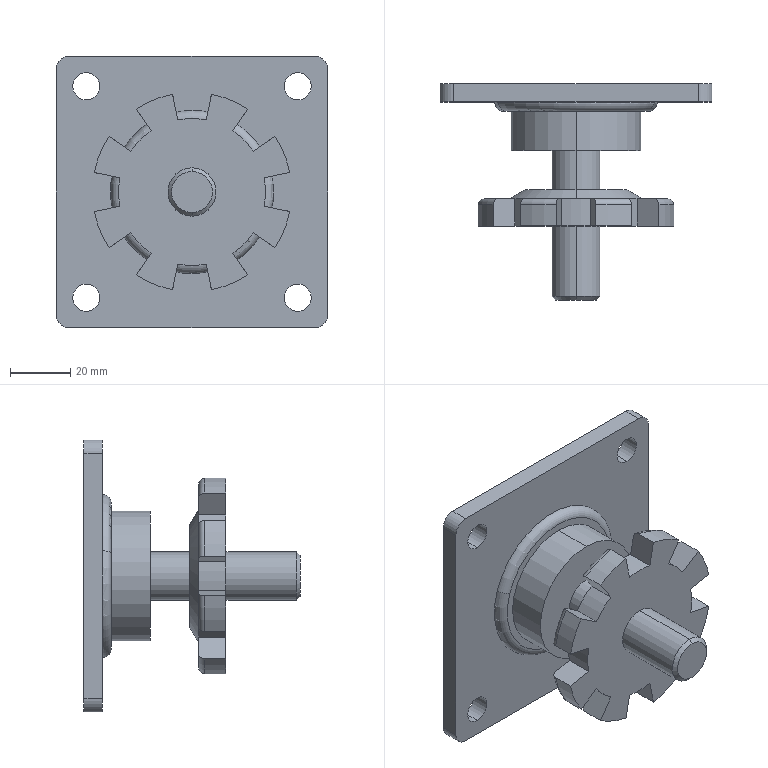Part | NX | features BREP 1 | 1 solid | 99 faces | box 90 x 71.5 x 90 mm | volume 104245 mm3 | plane 45 | cylinder 40 | torus 10 | cone 4 | commonest cylinder face diameters 9 x12 48.667 x8 66 x8 16 x6 10.667 x4 43 x2